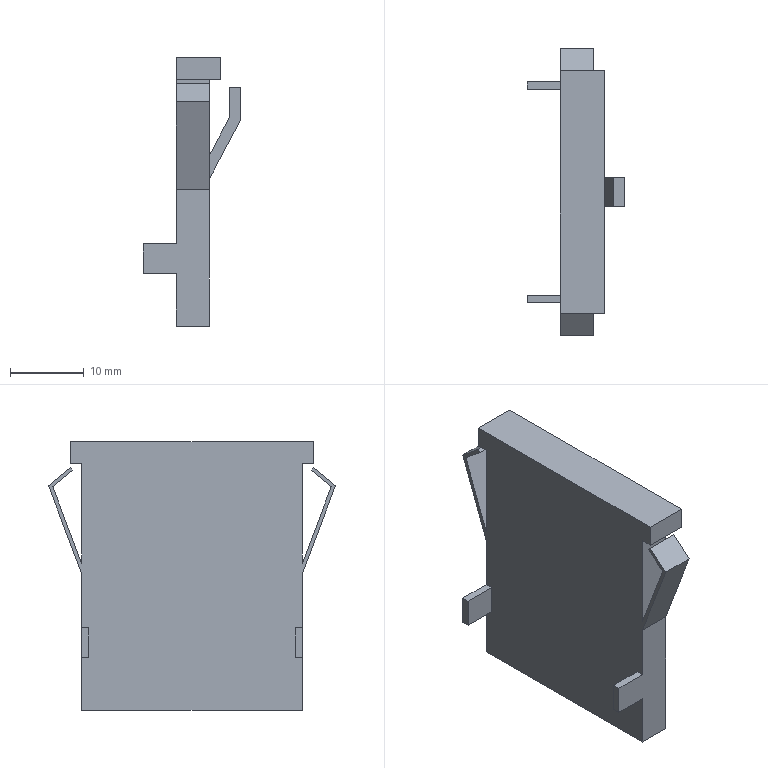Part | STEP file | A7P_M_RIGHT | 1 solid | 37 faces | box 13.3 x 39 x 36.5 mm | volume 5293 mm3 | plane 37
STEP:
#1=CARTESIAN_POINT('',(4.5,-15.,-14.9));
#2=VERTEX_POINT('',#1);
#3=CARTESIAN_POINT('',(4.5,-15.,-33.5));
#4=VERTEX_POINT('',#3);
#5=CARTESIAN_POINT('',(4.5,-15.,0.));
#6=DIRECTION('',(0.,0.,-1.));
#7=VECTOR('',#6,1000.);
#8=LINE('',#5,#7);
#9=EDGE_CURVE('',#2,#4,#8,.T.);
#10=ORIENTED_EDGE('',*,*,#9,.F.);
#11=CARTESIAN_POINT('',(0.,-15.,-14.9));
#12=VERTEX_POINT('',#11);
#13=CARTESIAN_POINT('',(0.,-15.,-14.9));
#14=DIRECTION('',(1.,0.,0.));
#15=VECTOR('',#14,1000.);
#16=LINE('',#13,#15);
#17=EDGE_CURVE('',#12,#2,#16,.T.);
#18=ORIENTED_EDGE('',*,*,#17,.F.);
#19=CARTESIAN_POINT('',(0.,-15.,-22.3));
#20=VERTEX_POINT('',#19);
#21=CARTESIAN_POINT('',(0.,-15.,0.));
#22=DIRECTION('',(0.,0.,-1.));
#23=VECTOR('',#22,1000.);
#24=LINE('',#21,#23);
#25=EDGE_CURVE('',#12,#20,#24,.T.);
#26=ORIENTED_EDGE('',*,*,#25,.T.);
#27=CARTESIAN_POINT('',(-4.5,-15.,-22.3));
#28=VERTEX_POINT('',#27);
#29=CARTESIAN_POINT('',(-4.5,-15.,-22.3));
#30=DIRECTION('',(1.,0.,0.));
#31=VECTOR('',#30,1000.);
#32=LINE('',#29,#31);
#33=EDGE_CURVE('',#28,#20,#32,.T.);
#34=ORIENTED_EDGE('',*,*,#33,.F.);
#35=CARTESIAN_POINT('',(-4.5,-15.,-26.3));
#36=VERTEX_POINT('',#35);
#37=CARTESIAN_POINT('',(-4.5,-15.,-22.3));
#38=DIRECTION('',(0.,0.,-1.));
#39=VECTOR('',#38,1000.);
#40=LINE('',#37,#39);
#41=EDGE_CURVE('',#28,#36,#40,.T.);
#42=ORIENTED_EDGE('',*,*,#41,.T.);
#43=CARTESIAN_POINT('',(0.,-15.,-26.3));
#44=VERTEX_POINT('',#43);
#45=CARTESIAN_POINT('',(-4.5,-15.,-26.3));
#46=DIRECTION('',(1.,0.,0.));
#47=VECTOR('',#46,1000.);
#48=LINE('',#45,#47);
#49=EDGE_CURVE('',#36,#44,#48,.T.);
#50=ORIENTED_EDGE('',*,*,#49,.T.);
#51=CARTESIAN_POINT('',(0.,-15.,-33.5));
#52=VERTEX_POINT('',#51);
#53=CARTESIAN_POINT('',(0.,-15.,0.));
#54=DIRECTION('',(0.,0.,-1.));
#55=VECTOR('',#54,1000.);
#56=LINE('',#53,#55);
#57=EDGE_CURVE('',#44,#52,#56,.T.);
#58=ORIENTED_EDGE('',*,*,#57,.T.);
#59=CARTESIAN_POINT('',(4.5,-15.,-33.5));
#60=DIRECTION('',(-1.,0.,0.));
#61=VECTOR('',#60,1000.);
#62=LINE('',#59,#61);
#63=EDGE_CURVE('',#4,#52,#62,.T.);
#64=ORIENTED_EDGE('',*,*,#63,.F.);
#65=EDGE_LOOP('',(#10,#18,#26,#34,#42,#50,#58,#64));
#66=FACE_OUTER_BOUND('',#65,.T.);
#67=CARTESIAN_POINT('',(4.5,-15.,0.));
#68=DIRECTION('',(0.,1.,0.));
#69=DIRECTION('',(0.,0.,1.));
#70=AXIS2_PLACEMENT_3D('',#67,#68,#69);
#71=PLANE('',#70);
#72=ADVANCED_FACE('',(#66),#71,.F.);
#73=CARTESIAN_POINT('',(0.,15.,-33.5));
#74=VERTEX_POINT('',#73);
#75=CARTESIAN_POINT('',(0.,15.,-26.3));
#76=VERTEX_POINT('',#75);
#77=CARTESIAN_POINT('',(0.,15.,0.));
#78=DIRECTION('',(0.,0.,1.));
#79=VECTOR('',#78,1000.);
#80=LINE('',#77,#79);
#81=EDGE_CURVE('',#74,#76,#80,.T.);
#82=ORIENTED_EDGE('',*,*,#81,.T.);
#83=CARTESIAN_POINT('',(-4.5,15.,-26.3));
#84=VERTEX_POINT('',#83);
#85=CARTESIAN_POINT('',(-4.5,15.,-26.3));
#86=DIRECTION('',(1.,0.,0.));
#87=VECTOR('',#86,1000.);
#88=LINE('',#85,#87);
#89=EDGE_CURVE('',#84,#76,#88,.T.);
#90=ORIENTED_EDGE('',*,*,#89,.F.);
#91=CARTESIAN_POINT('',(-4.5,15.,-22.3));
#92=VERTEX_POINT('',#91);
#93=CARTESIAN_POINT('',(-4.5,15.,-22.3));
#94=DIRECTION('',(0.,0.,1.));
#95=VECTOR('',#94,1000.);
#96=LINE('',#93,#95);
#97=EDGE_CURVE('',#84,#92,#96,.T.);
#98=ORIENTED_EDGE('',*,*,#97,.T.);
#99=CARTESIAN_POINT('',(0.,15.,-22.3));
#100=VERTEX_POINT('',#99);
#101=CARTESIAN_POINT('',(-4.5,15.,-22.3));
#102=DIRECTION('',(1.,0.,0.));
#103=VECTOR('',#102,1000.);
#104=LINE('',#101,#103);
#105=EDGE_CURVE('',#92,#100,#104,.T.);
#106=ORIENTED_EDGE('',*,*,#105,.T.);
#107=CARTESIAN_POINT('',(0.,15.,-14.9));
#108=VERTEX_POINT('',#107);
#109=CARTESIAN_POINT('',(0.,15.,0.));
#110=DIRECTION('',(0.,0.,1.));
#111=VECTOR('',#110,1000.);
#112=LINE('',#109,#111);
#113=EDGE_CURVE('',#100,#108,#112,.T.);
#114=ORIENTED_EDGE('',*,*,#113,.T.);
#115=CARTESIAN_POINT('',(4.5,15.,-14.9));
#116=VERTEX_POINT('',#115);
#117=CARTESIAN_POINT('',(0.,15.,-14.9));
#118=DIRECTION('',(1.,0.,0.));
#119=VECTOR('',#118,1000.);
#120=LINE('',#117,#119);
#121=EDGE_CURVE('',#108,#116,#120,.T.);
#122=ORIENTED_EDGE('',*,*,#121,.T.);
#123=CARTESIAN_POINT('',(4.5,15.,-33.5));
#124=VERTEX_POINT('',#123);
#125=CARTESIAN_POINT('',(4.5,15.,0.));
#126=DIRECTION('',(0.,0.,1.));
#127=VECTOR('',#126,1000.);
#128=LINE('',#125,#127);
#129=EDGE_CURVE('',#124,#116,#128,.T.);
#130=ORIENTED_EDGE('',*,*,#129,.F.);
#131=CARTESIAN_POINT('',(4.5,15.,-33.5));
#132=DIRECTION('',(-1.,0.,0.));
#133=VECTOR('',#132,1000.);
#134=LINE('',#131,#133);
#135=EDGE_CURVE('',#124,#74,#134,.T.);
#136=ORIENTED_EDGE('',*,*,#135,.T.);
#137=EDGE_LOOP('',(#82,#90,#98,#106,#114,#122,#130,#136));
#138=FACE_OUTER_BOUND('',#137,.T.);
#139=CARTESIAN_POINT('',(4.5,15.,0.));
#140=DIRECTION('',(0.,-1.,0.));
#141=DIRECTION('',(0.,0.,-1.));
#142=AXIS2_PLACEMENT_3D('',#139,#140,#141);
#143=PLANE('',#142);
#144=ADVANCED_FACE('',(#138),#143,.F.);
#145=ORIENTED_EDGE('',*,*,#129,.T.);
#146=CARTESIAN_POINT('',(4.5,19.5,-3.));
#147=VERTEX_POINT('',#146);
#148=CARTESIAN_POINT('',(4.5,19.5,-3.));
#149=DIRECTION('',(0.,0.3537,0.9354));
#150=VECTOR('',#149,1000.);
#151=LINE('',#148,#150);
#152=EDGE_CURVE('',#116,#147,#151,.T.);
#153=ORIENTED_EDGE('',*,*,#152,.T.);
#154=CARTESIAN_POINT('',(4.5,16.5,-0.5));
#155=VERTEX_POINT('',#154);
#156=CARTESIAN_POINT('',(4.5,16.5,-0.5));
#157=DIRECTION('',(0.,-0.7682,0.6402));
#158=VECTOR('',#157,1000.);
#159=LINE('',#156,#158);
#160=EDGE_CURVE('',#147,#155,#159,.T.);
#161=ORIENTED_EDGE('',*,*,#160,.T.);
#162=CARTESIAN_POINT('',(4.5,16.18,-0.8841));
#163=VERTEX_POINT('',#162);
#164=CARTESIAN_POINT('',(4.5,16.5,-0.5));
#165=DIRECTION('',(0.,-0.6402,-0.7682));
#166=VECTOR('',#165,1000.);
#167=LINE('',#164,#166);
#168=EDGE_CURVE('',#155,#163,#167,.T.);
#169=ORIENTED_EDGE('',*,*,#168,.T.);
#170=CARTESIAN_POINT('',(4.5,18.906,-3.156));
#171=VERTEX_POINT('',#170);
#172=CARTESIAN_POINT('',(4.5,16.18,-0.8841));
#173=DIRECTION('',(0.,0.7682,-0.6402));
#174=VECTOR('',#173,1000.);
#175=LINE('',#172,#174);
#176=EDGE_CURVE('',#163,#171,#175,.T.);
#177=ORIENTED_EDGE('',*,*,#176,.T.);
#178=CARTESIAN_POINT('',(4.5,15.,-13.486));
#179=VERTEX_POINT('',#178);
#180=CARTESIAN_POINT('',(4.5,18.906,-3.156));
#181=DIRECTION('',(0.,-0.3537,-0.9354));
#182=VECTOR('',#181,1000.);
#183=LINE('',#180,#182);
#184=EDGE_CURVE('',#171,#179,#183,.T.);
#185=ORIENTED_EDGE('',*,*,#184,.T.);
#186=CARTESIAN_POINT('',(4.5,15.,0.));
#187=VERTEX_POINT('',#186);
#188=CARTESIAN_POINT('',(4.5,15.,0.));
#189=DIRECTION('',(0.,0.,1.));
#190=VECTOR('',#189,1000.);
#191=LINE('',#188,#190);
#192=EDGE_CURVE('',#179,#187,#191,.T.);
#193=ORIENTED_EDGE('',*,*,#192,.T.);
#194=CARTESIAN_POINT('',(4.5,-15.,0.));
#195=VERTEX_POINT('',#194);
#196=CARTESIAN_POINT('',(4.5,16.5,0.));
#197=DIRECTION('',(0.,-1.,0.));
#198=VECTOR('',#197,1000.);
#199=LINE('',#196,#198);
#200=EDGE_CURVE('',#187,#195,#199,.T.);
#201=ORIENTED_EDGE('',*,*,#200,.T.);
#202=CARTESIAN_POINT('',(4.5,-15.,-13.486));
#203=VERTEX_POINT('',#202);
#204=CARTESIAN_POINT('',(4.5,-15.,0.));
#205=DIRECTION('',(0.,0.,-1.));
#206=VECTOR('',#205,1000.);
#207=LINE('',#204,#206);
#208=EDGE_CURVE('',#195,#203,#207,.T.);
#209=ORIENTED_EDGE('',*,*,#208,.T.);
#210=CARTESIAN_POINT('',(4.5,-18.906,-3.156));
#211=VERTEX_POINT('',#210);
#212=CARTESIAN_POINT('',(4.5,-18.906,-3.156));
#213=DIRECTION('',(0.,-0.3537,0.9354));
#214=VECTOR('',#213,1000.);
#215=LINE('',#212,#214);
#216=EDGE_CURVE('',#203,#211,#215,.T.);
#217=ORIENTED_EDGE('',*,*,#216,.T.);
#218=CARTESIAN_POINT('',(4.5,-16.18,-0.8841));
#219=VERTEX_POINT('',#218);
#220=CARTESIAN_POINT('',(4.5,-16.18,-0.8841));
#221=DIRECTION('',(0.,0.7682,0.6402));
#222=VECTOR('',#221,1000.);
#223=LINE('',#220,#222);
#224=EDGE_CURVE('',#211,#219,#223,.T.);
#225=ORIENTED_EDGE('',*,*,#224,.T.);
#226=CARTESIAN_POINT('',(4.5,-16.5,-0.5));
#227=VERTEX_POINT('',#226);
#228=CARTESIAN_POINT('',(4.5,-16.5,-0.5));
#229=DIRECTION('',(0.,-0.6402,0.7682));
#230=VECTOR('',#229,1000.);
#231=LINE('',#228,#230);
#232=EDGE_CURVE('',#219,#227,#231,.T.);
#233=ORIENTED_EDGE('',*,*,#232,.T.);
#234=CARTESIAN_POINT('',(4.5,-19.5,-3.));
#235=VERTEX_POINT('',#234);
#236=CARTESIAN_POINT('',(4.5,-16.5,-0.5));
#237=DIRECTION('',(0.,-0.7682,-0.6402));
#238=VECTOR('',#237,1000.);
#239=LINE('',#236,#238);
#240=EDGE_CURVE('',#227,#235,#239,.T.);
#241=ORIENTED_EDGE('',*,*,#240,.T.);
#242=CARTESIAN_POINT('',(4.5,-19.5,-3.));
#243=DIRECTION('',(0.,0.3537,-0.9354));
#244=VECTOR('',#243,1000.);
#245=LINE('',#242,#244);
#246=EDGE_CURVE('',#235,#2,#245,.T.);
#247=ORIENTED_EDGE('',*,*,#246,.T.);
#248=ORIENTED_EDGE('',*,*,#9,.T.);
#249=CARTESIAN_POINT('',(4.5,15.,-33.5));
#250=DIRECTION('',(0.,1.,0.));
#251=VECTOR('',#250,1000.);
#252=LINE('',#249,#251);
#253=EDGE_CURVE('',#4,#124,#252,.T.);
#254=ORIENTED_EDGE('',*,*,#253,.T.);
#255=EDGE_LOOP('',(#145,#153,#161,#169,#177,#185,#193,#201,#209,#217,#225,#233,#241,#247,#248,#254));
#256=FACE_OUTER_BOUND('',#255,.T.);
#257=CARTESIAN_POINT('',(4.5,2.,-10.292));
#258=VERTEX_POINT('',#257);
#259=CARTESIAN_POINT('',(4.5,-2.,-10.292));
#260=VERTEX_POINT('',#259);
#261=CARTESIAN_POINT('',(4.5,2.,-10.292));
#262=DIRECTION('',(0.,-1.,0.));
#263=VECTOR('',#262,1000.);
#264=LINE('',#261,#263);
#265=EDGE_CURVE('',#258,#260,#264,.T.);
#266=ORIENTED_EDGE('',*,*,#265,.F.);
#267=CARTESIAN_POINT('',(4.5,2.,-13.5));
#268=VERTEX_POINT('',#267);
#269=CARTESIAN_POINT('',(4.5,2.,-10.292));
#270=DIRECTION('',(0.,0.,1.));
#271=VECTOR('',#270,1000.);
#272=LINE('',#269,#271);
#273=EDGE_CURVE('',#268,#258,#272,.T.);
#274=ORIENTED_EDGE('',*,*,#273,.F.);
#275=CARTESIAN_POINT('',(4.5,-2.,-13.5));
#276=VERTEX_POINT('',#275);
#277=CARTESIAN_POINT('',(4.5,2.,-13.5));
#278=DIRECTION('',(0.,-1.,0.));
#279=VECTOR('',#278,1000.);
#280=LINE('',#277,#279);
#281=EDGE_CURVE('',#268,#276,#280,.T.);
#282=ORIENTED_EDGE('',*,*,#281,.T.);
#283=CARTESIAN_POINT('',(4.5,-2.,-10.292));
#284=DIRECTION('',(0.,0.,1.));
#285=VECTOR('',#284,1000.);
#286=LINE('',#283,#285);
#287=EDGE_CURVE('',#276,#260,#286,.T.);
#288=ORIENTED_EDGE('',*,*,#287,.T.);
#289=EDGE_LOOP('',(#266,#274,#282,#288));
#290=FACE_BOUND('',#289,.T.);
#291=CARTESIAN_POINT('',(4.5,16.5,0.));
#292=DIRECTION('',(1.,0.,0.));
#293=DIRECTION('',(0.,0.,-1.));
#294=AXIS2_PLACEMENT_3D('',#291,#292,#293);
#295=PLANE('',#294);
#296=ADVANCED_FACE('',(#256,#290),#295,.T.);
#297=CARTESIAN_POINT('',(0.,16.5,0.));
#298=VERTEX_POINT('',#297);
#299=CARTESIAN_POINT('',(0.,16.5,3.));
#300=VERTEX_POINT('',#299);
#301=CARTESIAN_POINT('',(0.,16.5,0.));
#302=DIRECTION('',(0.,0.,1.));
#303=VECTOR('',#302,1000.);
#304=LINE('',#301,#303);
#305=EDGE_CURVE('',#298,#300,#304,.T.);
#306=ORIENTED_EDGE('',*,*,#305,.T.);
#307=CARTESIAN_POINT('',(6.,16.5,3.));
#308=VERTEX_POINT('',#307);
#309=CARTESIAN_POINT('',(4.5,16.5,3.));
#310=DIRECTION('',(-1.,0.,0.));
#311=VECTOR('',#310,1000.);
#312=LINE('',#309,#311);
#313=EDGE_CURVE('',#308,#300,#312,.T.);
#314=ORIENTED_EDGE('',*,*,#313,.F.);
#315=CARTESIAN_POINT('',(6.,16.5,0.));
#316=VERTEX_POINT('',#315);
#317=CARTESIAN_POINT('',(6.,16.5,-33.541));
#318=DIRECTION('',(0.,0.,1.));
#319=VECTOR('',#318,1000.);
#320=LINE('',#317,#319);
#321=EDGE_CURVE('',#316,#308,#320,.T.);
#322=ORIENTED_EDGE('',*,*,#321,.F.);
#323=CARTESIAN_POINT('',(4.5,16.5,0.));
#324=DIRECTION('',(-1.,0.,0.));
#325=VECTOR('',#324,1000.);
#326=LINE('',#323,#325);
#327=EDGE_CURVE('',#316,#298,#326,.T.);
#328=ORIENTED_EDGE('',*,*,#327,.T.);
#329=EDGE_LOOP('',(#306,#314,#322,#328));
#330=FACE_OUTER_BOUND('',#329,.T.);
#331=CARTESIAN_POINT('',(4.5,16.5,0.));
#332=DIRECTION('',(0.,-1.,0.));
#333=DIRECTION('',(0.,0.,-1.));
#334=AXIS2_PLACEMENT_3D('',#331,#332,#333);
#335=PLANE('',#334);
#336=ADVANCED_FACE('',(#330),#335,.F.);
#337=CARTESIAN_POINT('',(0.,-16.5,3.));
#338=VERTEX_POINT('',#337);
#339=CARTESIAN_POINT('',(0.,16.5,3.));
#340=DIRECTION('',(0.,-1.,0.));
#341=VECTOR('',#340,1000.);
#342=LINE('',#339,#341);
#343=EDGE_CURVE('',#300,#338,#342,.T.);
#344=ORIENTED_EDGE('',*,*,#343,.T.);
#345=CARTESIAN_POINT('',(6.,-16.5,3.));
#346=VERTEX_POINT('',#345);
#347=CARTESIAN_POINT('',(4.5,-16.5,3.));
#348=DIRECTION('',(-1.,0.,0.));
#349=VECTOR('',#348,1000.);
#350=LINE('',#347,#349);
#351=EDGE_CURVE('',#346,#338,#350,.T.);
#352=ORIENTED_EDGE('',*,*,#351,.F.);
#353=CARTESIAN_POINT('',(6.,16.5,3.));
#354=DIRECTION('',(0.,1.,0.));
#355=VECTOR('',#354,1000.);
#356=LINE('',#353,#355);
#357=EDGE_CURVE('',#346,#308,#356,.T.);
#358=ORIENTED_EDGE('',*,*,#357,.T.);
#359=ORIENTED_EDGE('',*,*,#313,.T.);
#360=EDGE_LOOP('',(#344,#352,#358,#359));
#361=FACE_OUTER_BOUND('',#360,.T.);
#362=CARTESIAN_POINT('',(4.5,16.5,3.));
#363=DIRECTION('',(0.,0.,-1.));
#364=DIRECTION('',(-1.,0.,0.));
#365=AXIS2_PLACEMENT_3D('',#362,#363,#364);
#366=PLANE('',#365);
#367=ADVANCED_FACE('',(#361),#366,.F.);
#368=CARTESIAN_POINT('',(0.,-16.5,0.));
#369=VERTEX_POINT('',#368);
#370=CARTESIAN_POINT('',(0.,-16.5,3.));
#371=DIRECTION('',(0.,0.,-1.));
#372=VECTOR('',#371,1000.);
#373=LINE('',#370,#372);
#374=EDGE_CURVE('',#338,#369,#373,.T.);
#375=ORIENTED_EDGE('',*,*,#374,.T.);
#376=CARTESIAN_POINT('',(6.,-16.5,0.));
#377=VERTEX_POINT('',#376);
#378=CARTESIAN_POINT('',(4.5,-16.5,0.));
#379=DIRECTION('',(-1.,0.,0.));
#380=VECTOR('',#379,1000.);
#381=LINE('',#378,#380);
#382=EDGE_CURVE('',#377,#369,#381,.T.);
#383=ORIENTED_EDGE('',*,*,#382,.F.);
#384=CARTESIAN_POINT('',(6.,-16.5,-33.541));
#385=DIRECTION('',(0.,0.,1.));
#386=VECTOR('',#385,1000.);
#387=LINE('',#384,#386);
#388=EDGE_CURVE('',#377,#346,#387,.T.);
#389=ORIENTED_EDGE('',*,*,#388,.T.);
#390=ORIENTED_EDGE('',*,*,#351,.T.);
#391=EDGE_LOOP('',(#375,#383,#389,#390));
#392=FACE_OUTER_BOUND('',#391,.T.);
#393=CARTESIAN_POINT('',(4.5,-16.5,3.));
#394=DIRECTION('',(0.,1.,0.));
#395=DIRECTION('',(0.,0.,1.));
#396=AXIS2_PLACEMENT_3D('',#393,#394,#395);
#397=PLANE('',#396);
#398=ADVANCED_FACE('',(#392),#397,.F.);
#399=CARTESIAN_POINT('',(0.,-15.,0.));
#400=VERTEX_POINT('',#399);
#401=CARTESIAN_POINT('',(0.,-16.5,0.));
#402=DIRECTION('',(0.,1.,0.));
#403=VECTOR('',#402,1000.);
#404=LINE('',#401,#403);
#405=EDGE_CURVE('',#369,#400,#404,.T.);
#406=ORIENTED_EDGE('',*,*,#405,.T.);
#407=CARTESIAN_POINT('',(4.5,-15.,0.));
#408=DIRECTION('',(-1.,0.,0.));
#409=VECTOR('',#408,1000.);
#410=LINE('',#407,#409);
#411=EDGE_CURVE('',#195,#400,#410,.T.);
#412=ORIENTED_EDGE('',*,*,#411,.F.);
#413=ORIENTED_EDGE('',*,*,#200,.F.);
#414=CARTESIAN_POINT('',(0.,15.,0.));
#415=VERTEX_POINT('',#414);
#416=CARTESIAN_POINT('',(4.5,15.,0.));
#417=DIRECTION('',(-1.,0.,0.));
#418=VECTOR('',#417,1000.);
#419=LINE('',#416,#418);
#420=EDGE_CURVE('',#187,#415,#419,.T.);
#421=ORIENTED_EDGE('',*,*,#420,.T.);
#422=CARTESIAN_POINT('',(0.,15.,0.));
#423=DIRECTION('',(0.,1.,0.));
#424=VECTOR('',#423,1000.);
#425=LINE('',#422,#424);
#426=EDGE_CURVE('',#415,#298,#425,.T.);
#427=ORIENTED_EDGE('',*,*,#426,.T.);
#428=ORIENTED_EDGE('',*,*,#327,.F.);
#429=CARTESIAN_POINT('',(6.,16.5,0.));
#430=DIRECTION('',(0.,-1.,0.));
#431=VECTOR('',#430,1000.);
#432=LINE('',#429,#431);
#433=EDGE_CURVE('',#316,#377,#432,.T.);
#434=ORIENTED_EDGE('',*,*,#433,.T.);
#435=ORIENTED_EDGE('',*,*,#382,.T.);
#436=EDGE_LOOP('',(#406,#412,#413,#421,#427,#428,#434,#435));
#437=FACE_OUTER_BOUND('',#436,.T.);
#438=CARTESIAN_POINT('',(4.5,-16.5,0.));
#439=DIRECTION('',(0.,0.,1.));
#440=DIRECTION('',(1.,0.,0.));
#441=AXIS2_PLACEMENT_3D('',#438,#439,#440);
#442=PLANE('',#441);
#443=ADVANCED_FACE('',(#437),#442,.F.);
#444=CARTESIAN_POINT('',(0.,-15.,-13.486));
#445=VERTEX_POINT('',#444);
#446=CARTESIAN_POINT('',(0.,-15.,0.));
#447=DIRECTION('',(0.,0.,-1.));
#448=VECTOR('',#447,1000.);
#449=LINE('',#446,#448);
#450=EDGE_CURVE('',#400,#445,#449,.T.);
#451=ORIENTED_EDGE('',*,*,#450,.T.);
#452=CARTESIAN_POINT('',(0.,-15.,-13.486));
#453=DIRECTION('',(1.,0.,0.));
#454=VECTOR('',#453,1000.);
#455=LINE('',#452,#454);
#456=EDGE_CURVE('',#445,#203,#455,.T.);
#457=ORIENTED_EDGE('',*,*,#456,.T.);
#458=ORIENTED_EDGE('',*,*,#208,.F.);
#459=ORIENTED_EDGE('',*,*,#411,.T.);
#460=EDGE_LOOP('',(#451,#457,#458,#459));
#461=FACE_OUTER_BOUND('',#460,.T.);
#462=CARTESIAN_POINT('',(4.5,-15.,0.));
#463=DIRECTION('',(0.,1.,0.));
#464=DIRECTION('',(0.,0.,1.));
#465=AXIS2_PLACEMENT_3D('',#462,#463,#464);
#466=PLANE('',#465);
#467=ADVANCED_FACE('',(#461),#466,.F.);
#468=CARTESIAN_POINT('',(0.,15.,-33.5));
#469=DIRECTION('',(0.,1.,0.));
#470=VECTOR('',#469,1000.);
#471=LINE('',#468,#470);
#472=EDGE_CURVE('',#52,#74,#471,.T.);
#473=ORIENTED_EDGE('',*,*,#472,.T.);
#474=ORIENTED_EDGE('',*,*,#135,.F.);
#475=ORIENTED_EDGE('',*,*,#253,.F.);
#476=ORIENTED_EDGE('',*,*,#63,.T.);
#477=EDGE_LOOP('',(#473,#474,#475,#476));
#478=FACE_OUTER_BOUND('',#477,.T.);
#479=CARTESIAN_POINT('',(4.5,15.,-33.5));
#480=DIRECTION('',(0.,0.,1.));
#481=DIRECTION('',(1.,0.,0.));
#482=AXIS2_PLACEMENT_3D('',#479,#480,#481);
#483=PLANE('',#482);
#484=ADVANCED_FACE('',(#478),#483,.F.);
#485=ORIENTED_EDGE('',*,*,#192,.F.);
#486=CARTESIAN_POINT('',(0.,15.,-13.486));
#487=VERTEX_POINT('',#486);
#488=CARTESIAN_POINT('',(0.,15.,-13.486));
#489=DIRECTION('',(1.,0.,0.));
#490=VECTOR('',#489,1000.);
#491=LINE('',#488,#490);
#492=EDGE_CURVE('',#487,#179,#491,.T.);
#493=ORIENTED_EDGE('',*,*,#492,.F.);
#494=CARTESIAN_POINT('',(0.,15.,0.));
#495=DIRECTION('',(0.,0.,1.));
#496=VECTOR('',#495,1000.);
#497=LINE('',#494,#496);
#498=EDGE_CURVE('',#487,#415,#497,.T.);
#499=ORIENTED_EDGE('',*,*,#498,.T.);
#500=ORIENTED_EDGE('',*,*,#420,.F.);
#501=EDGE_LOOP('',(#485,#493,#499,#500));
#502=FACE_OUTER_BOUND('',#501,.T.);
#503=CARTESIAN_POINT('',(4.5,15.,0.));
#504=DIRECTION('',(0.,-1.,0.));
#505=DIRECTION('',(0.,0.,-1.));
#506=AXIS2_PLACEMENT_3D('',#503,#504,#505);
#507=PLANE('',#506);
#508=ADVANCED_FACE('',(#502),#507,.F.);
#509=CARTESIAN_POINT('',(0.,-14.,-26.3));
#510=VERTEX_POINT('',#509);
#511=CARTESIAN_POINT('',(0.,-14.,-22.3));
#512=VERTEX_POINT('',#511);
#513=CARTESIAN_POINT('',(0.,-14.,-22.3));
#514=DIRECTION('',(0.,0.,1.));
#515=VECTOR('',#514,1000.);
#516=LINE('',#513,#515);
#517=EDGE_CURVE('',#510,#512,#516,.T.);
#518=ORIENTED_EDGE('',*,*,#517,.T.);
#519=CARTESIAN_POINT('',(0.,-15.,-22.3));
#520=DIRECTION('',(0.,-1.,0.));
#521=VECTOR('',#520,1000.);
#522=LINE('',#519,#521);
#523=EDGE_CURVE('',#512,#20,#522,.T.);
#524=ORIENTED_EDGE('',*,*,#523,.T.);
#525=ORIENTED_EDGE('',*,*,#25,.F.);
#526=CARTESIAN_POINT('',(0.,-19.5,-3.));
#527=VERTEX_POINT('',#526);
#528=CARTESIAN_POINT('',(0.,-19.5,-3.));
#529=DIRECTION('',(0.,0.3537,-0.9354));
#530=VECTOR('',#529,1000.);
#531=LINE('',#528,#530);
#532=EDGE_CURVE('',#527,#12,#531,.T.);
#533=ORIENTED_EDGE('',*,*,#532,.F.);
#534=CARTESIAN_POINT('',(0.,-16.5,-0.5));
#535=VERTEX_POINT('',#534);
#536=CARTESIAN_POINT('',(0.,-16.5,-0.5));
#537=DIRECTION('',(0.,-0.7682,-0.6402));
#538=VECTOR('',#537,1000.);
#539=LINE('',#536,#538);
#540=EDGE_CURVE('',#535,#527,#539,.T.);
#541=ORIENTED_EDGE('',*,*,#540,.F.);
#542=CARTESIAN_POINT('',(0.,-16.18,-0.8841));
#543=VERTEX_POINT('',#542);
#544=CARTESIAN_POINT('',(0.,-16.5,-0.5));
#545=DIRECTION('',(0.,-0.6402,0.7682));
#546=VECTOR('',#545,1000.);
#547=LINE('',#544,#546);
#548=EDGE_CURVE('',#543,#535,#547,.T.);
#549=ORIENTED_EDGE('',*,*,#548,.F.);
#550=CARTESIAN_POINT('',(0.,-18.906,-3.156));
#551=VERTEX_POINT('',#550);
#552=CARTESIAN_POINT('',(0.,-16.18,-0.8841));
#553=DIRECTION('',(0.,0.7682,0.6402));
#554=VECTOR('',#553,1000.);
#555=LINE('',#552,#554);
#556=EDGE_CURVE('',#551,#543,#555,.T.);
#557=ORIENTED_EDGE('',*,*,#556,.F.);
#558=CARTESIAN_POINT('',(0.,-18.906,-3.156));
#559=DIRECTION('',(0.,-0.3537,0.9354));
#560=VECTOR('',#559,1000.);
#561=LINE('',#558,#560);
#562=EDGE_CURVE('',#445,#551,#561,.T.);
#563=ORIENTED_EDGE('',*,*,#562,.F.);
#564=ORIENTED_EDGE('',*,*,#450,.F.);
#565=ORIENTED_EDGE('',*,*,#405,.F.);
#566=ORIENTED_EDGE('',*,*,#374,.F.);
#567=ORIENTED_EDGE('',*,*,#343,.F.);
#568=ORIENTED_EDGE('',*,*,#305,.F.);
#569=ORIENTED_EDGE('',*,*,#426,.F.);
#570=ORIENTED_EDGE('',*,*,#498,.F.);
#571=CARTESIAN_POINT('',(0.,18.906,-3.156));
#572=VERTEX_POINT('',#571);
#573=CARTESIAN_POINT('',(0.,18.906,-3.156));
#574=DIRECTION('',(0.,-0.3537,-0.9354));
#575=VECTOR('',#574,1000.);
#576=LINE('',#573,#575);
#577=EDGE_CURVE('',#572,#487,#576,.T.);
#578=ORIENTED_EDGE('',*,*,#577,.F.);
#579=CARTESIAN_POINT('',(0.,16.18,-0.8841));
#580=VERTEX_POINT('',#579);
#581=CARTESIAN_POINT('',(0.,16.18,-0.8841));
#582=DIRECTION('',(0.,0.7682,-0.6402));
#583=VECTOR('',#582,1000.);
#584=LINE('',#581,#583);
#585=EDGE_CURVE('',#580,#572,#584,.T.);
#586=ORIENTED_EDGE('',*,*,#585,.F.);
#587=CARTESIAN_POINT('',(0.,16.5,-0.5));
#588=VERTEX_POINT('',#587);
#589=CARTESIAN_POINT('',(0.,16.5,-0.5));
#590=DIRECTION('',(0.,-0.6402,-0.7682));
#591=VECTOR('',#590,1000.);
#592=LINE('',#589,#591);
#593=EDGE_CURVE('',#588,#580,#592,.T.);
#594=ORIENTED_EDGE('',*,*,#593,.F.);
#595=CARTESIAN_POINT('',(0.,19.5,-3.));
#596=VERTEX_POINT('',#595);
#597=CARTESIAN_POINT('',(0.,16.5,-0.5));
#598=DIRECTION('',(0.,-0.7682,0.6402));
#599=VECTOR('',#598,1000.);
#600=LINE('',#597,#599);
#601=EDGE_CURVE('',#596,#588,#600,.T.);
#602=ORIENTED_EDGE('',*,*,#601,.F.);
#603=CARTESIAN_POINT('',(0.,19.5,-3.));
#604=DIRECTION('',(0.,0.3537,0.9354));
#605=VECTOR('',#604,1000.);
#606=LINE('',#603,#605);
#607=EDGE_CURVE('',#108,#596,#606,.T.);
#608=ORIENTED_EDGE('',*,*,#607,.F.);
#609=ORIENTED_EDGE('',*,*,#113,.F.);
#610=CARTESIAN_POINT('',(0.,14.,-22.3));
#611=VERTEX_POINT('',#610);
#612=CARTESIAN_POINT('',(0.,15.,-22.3));
#613=DIRECTION('',(0.,-1.,0.));
#614=VECTOR('',#613,1000.);
#615=LINE('',#612,#614);
#616=EDGE_CURVE('',#100,#611,#615,.T.);
#617=ORIENTED_EDGE('',*,*,#616,.T.);
#618=CARTESIAN_POINT('',(0.,14.,-26.3));
#619=VERTEX_POINT('',#618);
#620=CARTESIAN_POINT('',(0.,14.,-22.3));
#621=DIRECTION('',(0.,0.,-1.));
#622=VECTOR('',#621,1000.);
#623=LINE('',#620,#622);
#624=EDGE_CURVE('',#611,#619,#623,.T.);
#625=ORIENTED_EDGE('',*,*,#624,.T.);
#626=CARTESIAN_POINT('',(0.,15.,-26.3));
#627=DIRECTION('',(0.,1.,0.));
#628=VECTOR('',#627,1000.);
#629=LINE('',#626,#628);
#630=EDGE_CURVE('',#619,#76,#629,.T.);
#631=ORIENTED_EDGE('',*,*,#630,.T.);
#632=ORIENTED_EDGE('',*,*,#81,.F.);
#633=ORIENTED_EDGE('',*,*,#472,.F.);
#634=ORIENTED_EDGE('',*,*,#57,.F.);
#635=CARTESIAN_POINT('',(0.,-15.,-26.3));
#636=DIRECTION('',(0.,1.,0.));
#637=VECTOR('',#636,1000.);
#638=LINE('',#635,#637);
#639=EDGE_CURVE('',#44,#510,#638,.T.);
#640=ORIENTED_EDGE('',*,*,#639,.T.);
#641=EDGE_LOOP('',(#518,#524,#525,#533,#541,#549,#557,#563,#564,#565,#566,#567,#568,#569,#570,#578,#586,#594,#602,#608,#609,#617,#625,#631,#632,#633,#634,#640));
#642=FACE_OUTER_BOUND('',#641,.T.);
#643=CARTESIAN_POINT('',(0.,16.5,0.));
#644=DIRECTION('',(1.,0.,0.));
#645=DIRECTION('',(0.,0.,-1.));
#646=AXIS2_PLACEMENT_3D('',#643,#644,#645);
#647=PLANE('',#646);
#648=ADVANCED_FACE('',(#642),#647,.F.);
#649=ORIENTED_EDGE('',*,*,#433,.F.);
#650=ORIENTED_EDGE('',*,*,#321,.T.);
#651=ORIENTED_EDGE('',*,*,#357,.F.);
#652=ORIENTED_EDGE('',*,*,#388,.F.);
#653=EDGE_LOOP('',(#649,#650,#651,#652));
#654=FACE_OUTER_BOUND('',#653,.T.);
#655=CARTESIAN_POINT('',(6.,16.5,-33.541));
#656=DIRECTION('',(1.,0.,0.));
#657=DIRECTION('',(0.,1.,0.));
#658=AXIS2_PLACEMENT_3D('',#655,#656,#657);
#659=PLANE('',#658);
#660=ADVANCED_FACE('',(#654),#659,.T.);
#661=CARTESIAN_POINT('',(7.3,-2.,-5.));
#662=VERTEX_POINT('',#661);
#663=CARTESIAN_POINT('',(4.5,-2.,-10.292));
#664=DIRECTION('',(0.4676,0.,0.8839));
#665=VECTOR('',#664,1000.);
#666=LINE('',#663,#665);
#667=EDGE_CURVE('',#260,#662,#666,.T.);
#668=ORIENTED_EDGE('',*,*,#667,.T.);
#669=CARTESIAN_POINT('',(7.3,2.,-5.));
#670=VERTEX_POINT('',#669);
#671=CARTESIAN_POINT('',(7.3,2.,-5.));
#672=DIRECTION('',(0.,-1.,0.));
#673=VECTOR('',#672,1000.);
#674=LINE('',#671,#673);
#675=EDGE_CURVE('',#670,#662,#674,.T.);
#676=ORIENTED_EDGE('',*,*,#675,.F.);
#677=CARTESIAN_POINT('',(4.5,2.,-10.292));
#678=DIRECTION('',(0.4676,0.,0.8839));
#679=VECTOR('',#678,1000.);
#680=LINE('',#677,#679);
#681=EDGE_CURVE('',#258,#670,#680,.T.);
#682=ORIENTED_EDGE('',*,*,#681,.F.);
#683=ORIENTED_EDGE('',*,*,#265,.T.);
#684=EDGE_LOOP('',(#668,#676,#682,#683));
#685=FACE_OUTER_BOUND('',#684,.T.);
#686=CARTESIAN_POINT('',(4.5,2.,-10.292));
#687=DIRECTION('',(0.8839,0.,-0.4676));
#688=DIRECTION('',(-0.4676,0.,-0.8839));
#689=AXIS2_PLACEMENT_3D('',#686,#687,#688);
#690=PLANE('',#689);
#691=ADVANCED_FACE('',(#685),#690,.F.);
#692=CARTESIAN_POINT('',(7.3,-2.,-1.));
#693=VERTEX_POINT('',#692);
#694=CARTESIAN_POINT('',(7.3,-2.,-5.));
#695=DIRECTION('',(0.,0.,1.));
#696=VECTOR('',#695,1000.);
#697=LINE('',#694,#696);
#698=EDGE_CURVE('',#662,#693,#697,.T.);
#699=ORIENTED_EDGE('',*,*,#698,.T.);
#700=CARTESIAN_POINT('',(7.3,2.,-1.));
#701=VERTEX_POINT('',#700);
#702=CARTESIAN_POINT('',(7.3,2.,-1.));
#703=DIRECTION('',(0.,-1.,0.));
#704=VECTOR('',#703,1000.);
#705=LINE('',#702,#704);
#706=EDGE_CURVE('',#701,#693,#705,.T.);
#707=ORIENTED_EDGE('',*,*,#706,.F.);
#708=CARTESIAN_POINT('',(7.3,2.,-5.));
#709=DIRECTION('',(0.,0.,1.));
#710=VECTOR('',#709,1000.);
#711=LINE('',#708,#710);
#712=EDGE_CURVE('',#670,#701,#711,.T.);
#713=ORIENTED_EDGE('',*,*,#712,.F.);
#714=ORIENTED_EDGE('',*,*,#675,.T.);
#715=EDGE_LOOP('',(#699,#707,#713,#714));
#716=FACE_OUTER_BOUND('',#715,.T.);
#717=CARTESIAN_POINT('',(7.3,2.,-5.));
#718=DIRECTION('',(1.,0.,0.));
#719=DIRECTION('',(0.,0.,-1.));
#720=AXIS2_PLACEMENT_3D('',#717,#718,#719);
#721=PLANE('',#720);
#722=ADVANCED_FACE('',(#716),#721,.F.);
#723=CARTESIAN_POINT('',(8.8,-2.,-1.));
#724=VERTEX_POINT('',#723);
#725=CARTESIAN_POINT('',(7.3,-2.,-1.));
#726=DIRECTION('',(1.,0.,0.));
#727=VECTOR('',#726,1000.);
#728=LINE('',#725,#727);
#729=EDGE_CURVE('',#693,#724,#728,.T.);
#730=ORIENTED_EDGE('',*,*,#729,.T.);
#731=CARTESIAN_POINT('',(8.8,2.,-1.));
#732=VERTEX_POINT('',#731);
#733=CARTESIAN_POINT('',(8.8,2.,-1.));
#734=DIRECTION('',(0.,-1.,0.));
#735=VECTOR('',#734,1000.);
#736=LINE('',#733,#735);
#737=EDGE_CURVE('',#732,#724,#736,.T.);
#738=ORIENTED_EDGE('',*,*,#737,.F.);
#739=CARTESIAN_POINT('',(7.3,2.,-1.));
#740=DIRECTION('',(1.,0.,0.));
#741=VECTOR('',#740,1000.);
#742=LINE('',#739,#741);
#743=EDGE_CURVE('',#701,#732,#742,.T.);
#744=ORIENTED_EDGE('',*,*,#743,.F.);
#745=ORIENTED_EDGE('',*,*,#706,.T.);
#746=EDGE_LOOP('',(#730,#738,#744,#745));
#747=FACE_OUTER_BOUND('',#746,.T.);
#748=CARTESIAN_POINT('',(7.3,2.,-1.));
#749=DIRECTION('',(0.,0.,-1.));
#750=DIRECTION('',(-1.,0.,0.));
#751=AXIS2_PLACEMENT_3D('',#748,#749,#750);
#752=PLANE('',#751);
#753=ADVANCED_FACE('',(#747),#752,.F.);
#754=CARTESIAN_POINT('',(8.8,-2.,-5.372));
#755=VERTEX_POINT('',#754);
#756=CARTESIAN_POINT('',(8.8,-2.,-5.372));
#757=DIRECTION('',(0.,0.,-1.));
#758=VECTOR('',#757,1000.);
#759=LINE('',#756,#758);
#760=EDGE_CURVE('',#724,#755,#759,.T.);
#761=ORIENTED_EDGE('',*,*,#760,.T.);
#762=CARTESIAN_POINT('',(8.8,2.,-5.372));
#763=VERTEX_POINT('',#762);
#764=CARTESIAN_POINT('',(8.8,2.,-5.372));
#765=DIRECTION('',(0.,-1.,0.));
#766=VECTOR('',#765,1000.);
#767=LINE('',#764,#766);
#768=EDGE_CURVE('',#763,#755,#767,.T.);
#769=ORIENTED_EDGE('',*,*,#768,.F.);
#770=CARTESIAN_POINT('',(8.8,2.,-5.372));
#771=DIRECTION('',(0.,0.,-1.));
#772=VECTOR('',#771,1000.);
#773=LINE('',#770,#772);
#774=EDGE_CURVE('',#732,#763,#773,.T.);
#775=ORIENTED_EDGE('',*,*,#774,.F.);
#776=ORIENTED_EDGE('',*,*,#737,.T.);
#777=EDGE_LOOP('',(#761,#769,#775,#776));
#778=FACE_OUTER_BOUND('',#777,.T.);
#779=CARTESIAN_POINT('',(8.8,2.,-5.372));
#780=DIRECTION('',(-1.,0.,0.));
#781=DIRECTION('',(0.,0.,1.));
#782=AXIS2_PLACEMENT_3D('',#779,#780,#781);
#783=PLANE('',#782);
#784=ADVANCED_FACE('',(#778),#783,.F.);
#785=CARTESIAN_POINT('',(4.5,-2.,-13.5));
#786=DIRECTION('',(-0.4676,0.,-0.8839));
#787=VECTOR('',#786,1000.);
#788=LINE('',#785,#787);
#789=EDGE_CURVE('',#755,#276,#788,.T.);
#790=ORIENTED_EDGE('',*,*,#789,.T.);
#791=ORIENTED_EDGE('',*,*,#281,.F.);
#792=CARTESIAN_POINT('',(4.5,2.,-13.5));
#793=DIRECTION('',(-0.4676,0.,-0.8839));
#794=VECTOR('',#793,1000.);
#795=LINE('',#792,#794);
#796=EDGE_CURVE('',#763,#268,#795,.T.);
#797=ORIENTED_EDGE('',*,*,#796,.F.);
#798=ORIENTED_EDGE('',*,*,#768,.T.);
#799=EDGE_LOOP('',(#790,#791,#797,#798));
#800=FACE_OUTER_BOUND('',#799,.T.);
#801=CARTESIAN_POINT('',(4.5,2.,-13.5));
#802=DIRECTION('',(-0.8839,0.,0.4676));
#803=DIRECTION('',(0.4676,0.,0.8839));
#804=AXIS2_PLACEMENT_3D('',#801,#802,#803);
#805=PLANE('',#804);
#806=ADVANCED_FACE('',(#800),#805,.F.);
#807=ORIENTED_EDGE('',*,*,#273,.T.);
#808=ORIENTED_EDGE('',*,*,#681,.T.);
#809=ORIENTED_EDGE('',*,*,#712,.T.);
#810=ORIENTED_EDGE('',*,*,#743,.T.);
#811=ORIENTED_EDGE('',*,*,#774,.T.);
#812=ORIENTED_EDGE('',*,*,#796,.T.);
#813=EDGE_LOOP('',(#807,#808,#809,#810,#811,#812));
#814=FACE_OUTER_BOUND('',#813,.T.);
#815=CARTESIAN_POINT('',(4.5,2.,-1.));
#816=DIRECTION('',(0.,-1.,0.));
#817=DIRECTION('',(0.,0.,-1.));
#818=AXIS2_PLACEMENT_3D('',#815,#816,#817);
#819=PLANE('',#818);
#820=ADVANCED_FACE('',(#814),#819,.F.);
#821=ORIENTED_EDGE('',*,*,#287,.F.);
#822=ORIENTED_EDGE('',*,*,#789,.F.);
#823=ORIENTED_EDGE('',*,*,#760,.F.);
#824=ORIENTED_EDGE('',*,*,#729,.F.);
#825=ORIENTED_EDGE('',*,*,#698,.F.);
#826=ORIENTED_EDGE('',*,*,#667,.F.);
#827=EDGE_LOOP('',(#821,#822,#823,#824,#825,#826));
#828=FACE_OUTER_BOUND('',#827,.T.);
#829=CARTESIAN_POINT('',(4.5,-2.,-1.));
#830=DIRECTION('',(0.,-1.,0.));
#831=DIRECTION('',(0.,0.,-1.));
#832=AXIS2_PLACEMENT_3D('',#829,#830,#831);
#833=PLANE('',#832);
#834=ADVANCED_FACE('',(#828),#833,.T.);
#835=ORIENTED_EDGE('',*,*,#168,.F.);
#836=CARTESIAN_POINT('',(0.,16.5,-0.5));
#837=DIRECTION('',(1.,0.,0.));
#838=VECTOR('',#837,1000.);
#839=LINE('',#836,#838);
#840=EDGE_CURVE('',#588,#155,#839,.T.);
#841=ORIENTED_EDGE('',*,*,#840,.F.);
#842=ORIENTED_EDGE('',*,*,#593,.T.);
#843=CARTESIAN_POINT('',(0.,16.18,-0.8841));
#844=DIRECTION('',(1.,0.,0.));
#845=VECTOR('',#844,1000.);
#846=LINE('',#843,#845);
#847=EDGE_CURVE('',#580,#163,#846,.T.);
#848=ORIENTED_EDGE('',*,*,#847,.T.);
#849=EDGE_LOOP('',(#835,#841,#842,#848));
#850=FACE_OUTER_BOUND('',#849,.T.);
#851=CARTESIAN_POINT('',(0.,16.5,-0.5));
#852=DIRECTION('',(0.,-0.7682,0.6402));
#853=DIRECTION('',(0.,-0.6402,-0.7682));
#854=AXIS2_PLACEMENT_3D('',#851,#852,#853);
#855=PLANE('',#854);
#856=ADVANCED_FACE('',(#850),#855,.T.);
#857=ORIENTED_EDGE('',*,*,#160,.F.);
#858=CARTESIAN_POINT('',(0.,19.5,-3.));
#859=DIRECTION('',(1.,0.,0.));
#860=VECTOR('',#859,1000.);
#861=LINE('',#858,#860);
#862=EDGE_CURVE('',#596,#147,#861,.T.);
#863=ORIENTED_EDGE('',*,*,#862,.F.);
#864=ORIENTED_EDGE('',*,*,#601,.T.);
#865=ORIENTED_EDGE('',*,*,#840,.T.);
#866=EDGE_LOOP('',(#857,#863,#864,#865));
#867=FACE_OUTER_BOUND('',#866,.T.);
#868=CARTESIAN_POINT('',(0.,16.5,-0.5));
#869=DIRECTION('',(0.,0.6402,0.7682));
#870=DIRECTION('',(0.,-0.7682,0.6402));
#871=AXIS2_PLACEMENT_3D('',#868,#869,#870);
#872=PLANE('',#871);
#873=ADVANCED_FACE('',(#867),#872,.T.);
#874=ORIENTED_EDGE('',*,*,#152,.F.);
#875=ORIENTED_EDGE('',*,*,#121,.F.);
#876=ORIENTED_EDGE('',*,*,#607,.T.);
#877=ORIENTED_EDGE('',*,*,#862,.T.);
#878=EDGE_LOOP('',(#874,#875,#876,#877));
#879=FACE_OUTER_BOUND('',#878,.T.);
#880=CARTESIAN_POINT('',(0.,19.5,-3.));
#881=DIRECTION('',(0.,0.9354,-0.3537));
#882=DIRECTION('',(0.,0.3537,0.9354));
#883=AXIS2_PLACEMENT_3D('',#880,#881,#882);
#884=PLANE('',#883);
#885=ADVANCED_FACE('',(#879),#884,.T.);
#886=ORIENTED_EDGE('',*,*,#184,.F.);
#887=CARTESIAN_POINT('',(0.,18.906,-3.156));
#888=DIRECTION('',(1.,0.,0.));
#889=VECTOR('',#888,1000.);
#890=LINE('',#887,#889);
#891=EDGE_CURVE('',#572,#171,#890,.T.);
#892=ORIENTED_EDGE('',*,*,#891,.F.);
#893=ORIENTED_EDGE('',*,*,#577,.T.);
#894=ORIENTED_EDGE('',*,*,#492,.T.);
#895=EDGE_LOOP('',(#886,#892,#893,#894));
#896=FACE_OUTER_BOUND('',#895,.T.);
#897=CARTESIAN_POINT('',(0.,18.906,-3.156));
#898=DIRECTION('',(0.,-0.9354,0.3537));
#899=DIRECTION('',(0.,-0.3537,-0.9354));
#900=AXIS2_PLACEMENT_3D('',#897,#898,#899);
#901=PLANE('',#900);
#902=ADVANCED_FACE('',(#896),#901,.T.);
#903=ORIENTED_EDGE('',*,*,#176,.F.);
#904=ORIENTED_EDGE('',*,*,#847,.F.);
#905=ORIENTED_EDGE('',*,*,#585,.T.);
#906=ORIENTED_EDGE('',*,*,#891,.T.);
#907=EDGE_LOOP('',(#903,#904,#905,#906));
#908=FACE_OUTER_BOUND('',#907,.T.);
#909=CARTESIAN_POINT('',(0.,16.18,-0.8841));
#910=DIRECTION('',(0.,-0.6402,-0.7682));
#911=DIRECTION('',(0.,0.7682,-0.6402));
#912=AXIS2_PLACEMENT_3D('',#909,#910,#911);
#913=PLANE('',#912);
#914=ADVANCED_FACE('',(#908),#913,.T.);
#915=ORIENTED_EDGE('',*,*,#246,.F.);
#916=CARTESIAN_POINT('',(0.,-19.5,-3.));
#917=DIRECTION('',(1.,0.,0.));
#918=VECTOR('',#917,1000.);
#919=LINE('',#916,#918);
#920=EDGE_CURVE('',#527,#235,#919,.T.);
#921=ORIENTED_EDGE('',*,*,#920,.F.);
#922=ORIENTED_EDGE('',*,*,#532,.T.);
#923=ORIENTED_EDGE('',*,*,#17,.T.);
#924=EDGE_LOOP('',(#915,#921,#922,#923));
#925=FACE_OUTER_BOUND('',#924,.T.);
#926=CARTESIAN_POINT('',(0.,-19.5,-3.));
#927=DIRECTION('',(0.,-0.9354,-0.3537));
#928=DIRECTION('',(0.,0.3537,-0.9354));
#929=AXIS2_PLACEMENT_3D('',#926,#927,#928);
#930=PLANE('',#929);
#931=ADVANCED_FACE('',(#925),#930,.T.);
#932=ORIENTED_EDGE('',*,*,#240,.F.);
#933=CARTESIAN_POINT('',(0.,-16.5,-0.5));
#934=DIRECTION('',(1.,0.,0.));
#935=VECTOR('',#934,1000.);
#936=LINE('',#933,#935);
#937=EDGE_CURVE('',#535,#227,#936,.T.);
#938=ORIENTED_EDGE('',*,*,#937,.F.);
#939=ORIENTED_EDGE('',*,*,#540,.T.);
#940=ORIENTED_EDGE('',*,*,#920,.T.);
#941=EDGE_LOOP('',(#932,#938,#939,#940));
#942=FACE_OUTER_BOUND('',#941,.T.);
#943=CARTESIAN_POINT('',(0.,-16.5,-0.5));
#944=DIRECTION('',(0.,-0.6402,0.7682));
#945=DIRECTION('',(0.,-0.7682,-0.6402));
#946=AXIS2_PLACEMENT_3D('',#943,#944,#945);
#947=PLANE('',#946);
#948=ADVANCED_FACE('',(#942),#947,.T.);
#949=ORIENTED_EDGE('',*,*,#232,.F.);
#950=CARTESIAN_POINT('',(0.,-16.18,-0.8841));
#951=DIRECTION('',(1.,0.,0.));
#952=VECTOR('',#951,1000.);
#953=LINE('',#950,#952);
#954=EDGE_CURVE('',#543,#219,#953,.T.);
#955=ORIENTED_EDGE('',*,*,#954,.F.);
#956=ORIENTED_EDGE('',*,*,#548,.T.);
#957=ORIENTED_EDGE('',*,*,#937,.T.);
#958=EDGE_LOOP('',(#949,#955,#956,#957));
#959=FACE_OUTER_BOUND('',#958,.T.);
#960=CARTESIAN_POINT('',(0.,-16.5,-0.5));
#961=DIRECTION('',(0.,0.7682,0.6402));
#962=DIRECTION('',(0.,-0.6402,0.7682));
#963=AXIS2_PLACEMENT_3D('',#960,#961,#962);
#964=PLANE('',#963);
#965=ADVANCED_FACE('',(#959),#964,.T.);
#966=ORIENTED_EDGE('',*,*,#224,.F.);
#967=CARTESIAN_POINT('',(0.,-18.906,-3.156));
#968=DIRECTION('',(1.,0.,0.));
#969=VECTOR('',#968,1000.);
#970=LINE('',#967,#969);
#971=EDGE_CURVE('',#551,#211,#970,.T.);
#972=ORIENTED_EDGE('',*,*,#971,.F.);
#973=ORIENTED_EDGE('',*,*,#556,.T.);
#974=ORIENTED_EDGE('',*,*,#954,.T.);
#975=EDGE_LOOP('',(#966,#972,#973,#974));
#976=FACE_OUTER_BOUND('',#975,.T.);
#977=CARTESIAN_POINT('',(0.,-16.18,-0.8841));
#978=DIRECTION('',(0.,0.6402,-0.7682));
#979=DIRECTION('',(0.,0.7682,0.6402));
#980=AXIS2_PLACEMENT_3D('',#977,#978,#979);
#981=PLANE('',#980);
#982=ADVANCED_FACE('',(#976),#981,.T.);
#983=ORIENTED_EDGE('',*,*,#216,.F.);
#984=ORIENTED_EDGE('',*,*,#456,.F.);
#985=ORIENTED_EDGE('',*,*,#562,.T.);
#986=ORIENTED_EDGE('',*,*,#971,.T.);
#987=EDGE_LOOP('',(#983,#984,#985,#986));
#988=FACE_OUTER_BOUND('',#987,.T.);
#989=CARTESIAN_POINT('',(0.,-18.906,-3.156));
#990=DIRECTION('',(0.,0.9354,0.3537));
#991=DIRECTION('',(0.,-0.3537,0.9354));
#992=AXIS2_PLACEMENT_3D('',#989,#990,#991);
#993=PLANE('',#992);
#994=ADVANCED_FACE('',(#988),#993,.T.);
#995=ORIENTED_EDGE('',*,*,#616,.F.);
#996=ORIENTED_EDGE('',*,*,#105,.F.);
#997=CARTESIAN_POINT('',(-4.5,14.,-22.3));
#998=VERTEX_POINT('',#997);
#999=CARTESIAN_POINT('',(-4.5,15.,-22.3));
#1000=DIRECTION('',(0.,-1.,0.));
#1001=VECTOR('',#1000,1000.);
#1002=LINE('',#999,#1001);
#1003=EDGE_CURVE('',#92,#998,#1002,.T.);
#1004=ORIENTED_EDGE('',*,*,#1003,.T.);
#1005=CARTESIAN_POINT('',(-4.5,14.,-22.3));
#1006=DIRECTION('',(1.,0.,0.));
#1007=VECTOR('',#1006,1000.);
#1008=LINE('',#1005,#1007);
#1009=EDGE_CURVE('',#998,#611,#1008,.T.);
#1010=ORIENTED_EDGE('',*,*,#1009,.T.);
#1011=EDGE_LOOP('',(#995,#996,#1004,#1010));
#1012=FACE_OUTER_BOUND('',#1011,.T.);
#1013=CARTESIAN_POINT('',(-4.5,15.,-22.3));
#1014=DIRECTION('',(0.,0.,1.));
#1015=DIRECTION('',(0.,-1.,0.));
#1016=AXIS2_PLACEMENT_3D('',#1013,#1014,#1015);
#1017=PLANE('',#1016);
#1018=ADVANCED_FACE('',(#1012),#1017,.T.);
#1019=ORIENTED_EDGE('',*,*,#630,.F.);
#1020=CARTESIAN_POINT('',(-4.5,14.,-26.3));
#1021=VERTEX_POINT('',#1020);
#1022=CARTESIAN_POINT('',(-4.5,14.,-26.3));
#1023=DIRECTION('',(1.,0.,0.));
#1024=VECTOR('',#1023,1000.);
#1025=LINE('',#1022,#1024);
#1026=EDGE_CURVE('',#1021,#619,#1025,.T.);
#1027=ORIENTED_EDGE('',*,*,#1026,.F.);
#1028=CARTESIAN_POINT('',(-4.5,15.,-26.3));
#1029=DIRECTION('',(0.,1.,0.));
#1030=VECTOR('',#1029,1000.);
#1031=LINE('',#1028,#1030);
#1032=EDGE_CURVE('',#1021,#84,#1031,.T.);
#1033=ORIENTED_EDGE('',*,*,#1032,.T.);
#1034=ORIENTED_EDGE('',*,*,#89,.T.);
#1035=EDGE_LOOP('',(#1019,#1027,#1033,#1034));
#1036=FACE_OUTER_BOUND('',#1035,.T.);
#1037=CARTESIAN_POINT('',(-4.5,15.,-26.3));
#1038=DIRECTION('',(0.,0.,-1.));
#1039=DIRECTION('',(0.,1.,0.));
#1040=AXIS2_PLACEMENT_3D('',#1037,#1038,#1039);
#1041=PLANE('',#1040);
#1042=ADVANCED_FACE('',(#1036),#1041,.T.);
#1043=ORIENTED_EDGE('',*,*,#624,.F.);
#1044=ORIENTED_EDGE('',*,*,#1009,.F.);
#1045=CARTESIAN_POINT('',(-4.5,14.,-22.3));
#1046=DIRECTION('',(0.,0.,-1.));
#1047=VECTOR('',#1046,1000.);
#1048=LINE('',#1045,#1047);
#1049=EDGE_CURVE('',#998,#1021,#1048,.T.);
#1050=ORIENTED_EDGE('',*,*,#1049,.T.);
#1051=ORIENTED_EDGE('',*,*,#1026,.T.);
#1052=EDGE_LOOP('',(#1043,#1044,#1050,#1051));
#1053=FACE_OUTER_BOUND('',#1052,.T.);
#1054=CARTESIAN_POINT('',(-4.5,14.,-22.3));
#1055=DIRECTION('',(0.,-1.,0.));
#1056=DIRECTION('',(0.,0.,-1.));
#1057=AXIS2_PLACEMENT_3D('',#1054,#1055,#1056);
#1058=PLANE('',#1057);
#1059=ADVANCED_FACE('',(#1053),#1058,.T.);
#1060=ORIENTED_EDGE('',*,*,#1003,.F.);
#1061=ORIENTED_EDGE('',*,*,#97,.F.);
#1062=ORIENTED_EDGE('',*,*,#1032,.F.);
#1063=ORIENTED_EDGE('',*,*,#1049,.F.);
#1064=EDGE_LOOP('',(#1060,#1061,#1062,#1063));
#1065=FACE_OUTER_BOUND('',#1064,.T.);
#1066=CARTESIAN_POINT('',(-4.5,14.,-22.3));
#1067=DIRECTION('',(1.,0.,0.));
#1068=DIRECTION('',(0.,0.,-1.));
#1069=AXIS2_PLACEMENT_3D('',#1066,#1067,#1068);
#1070=PLANE('',#1069);
#1071=ADVANCED_FACE('',(#1065),#1070,.F.);
#1072=ORIENTED_EDGE('',*,*,#523,.F.);
#1073=CARTESIAN_POINT('',(-4.5,-14.,-22.3));
#1074=VERTEX_POINT('',#1073);
#1075=CARTESIAN_POINT('',(-4.5,-14.,-22.3));
#1076=DIRECTION('',(1.,0.,0.));
#1077=VECTOR('',#1076,1000.);
#1078=LINE('',#1075,#1077);
#1079=EDGE_CURVE('',#1074,#512,#1078,.T.);
#1080=ORIENTED_EDGE('',*,*,#1079,.F.);
#1081=CARTESIAN_POINT('',(-4.5,-15.,-22.3));
#1082=DIRECTION('',(0.,-1.,0.));
#1083=VECTOR('',#1082,1000.);
#1084=LINE('',#1081,#1083);
#1085=EDGE_CURVE('',#1074,#28,#1084,.T.);
#1086=ORIENTED_EDGE('',*,*,#1085,.T.);
#1087=ORIENTED_EDGE('',*,*,#33,.T.);
#1088=EDGE_LOOP('',(#1072,#1080,#1086,#1087));
#1089=FACE_OUTER_BOUND('',#1088,.T.);
#1090=CARTESIAN_POINT('',(-4.5,-15.,-22.3));
#1091=DIRECTION('',(0.,0.,1.));
#1092=DIRECTION('',(0.,-1.,0.));
#1093=AXIS2_PLACEMENT_3D('',#1090,#1091,#1092);
#1094=PLANE('',#1093);
#1095=ADVANCED_FACE('',(#1089),#1094,.T.);
#1096=ORIENTED_EDGE('',*,*,#517,.F.);
#1097=CARTESIAN_POINT('',(-4.5,-14.,-26.3));
#1098=VERTEX_POINT('',#1097);
#1099=CARTESIAN_POINT('',(-4.5,-14.,-26.3));
#1100=DIRECTION('',(1.,0.,0.));
#1101=VECTOR('',#1100,1000.);
#1102=LINE('',#1099,#1101);
#1103=EDGE_CURVE('',#1098,#510,#1102,.T.);
#1104=ORIENTED_EDGE('',*,*,#1103,.F.);
#1105=CARTESIAN_POINT('',(-4.5,-14.,-22.3));
#1106=DIRECTION('',(0.,0.,1.));
#1107=VECTOR('',#1106,1000.);
#1108=LINE('',#1105,#1107);
#1109=EDGE_CURVE('',#1098,#1074,#1108,.T.);
#1110=ORIENTED_EDGE('',*,*,#1109,.T.);
#1111=ORIENTED_EDGE('',*,*,#1079,.T.);
#1112=EDGE_LOOP('',(#1096,#1104,#1110,#1111));
#1113=FACE_OUTER_BOUND('',#1112,.T.);
#1114=CARTESIAN_POINT('',(-4.5,-14.,-22.3));
#1115=DIRECTION('',(0.,1.,0.));
#1116=DIRECTION('',(0.,0.,1.));
#1117=AXIS2_PLACEMENT_3D('',#1114,#1115,#1116);
#1118=PLANE('',#1117);
#1119=ADVANCED_FACE('',(#1113),#1118,.T.);
#1120=ORIENTED_EDGE('',*,*,#639,.F.);
#1121=ORIENTED_EDGE('',*,*,#49,.F.);
#1122=CARTESIAN_POINT('',(-4.5,-15.,-26.3));
#1123=DIRECTION('',(0.,1.,0.));
#1124=VECTOR('',#1123,1000.);
#1125=LINE('',#1122,#1124);
#1126=EDGE_CURVE('',#36,#1098,#1125,.T.);
#1127=ORIENTED_EDGE('',*,*,#1126,.T.);
#1128=ORIENTED_EDGE('',*,*,#1103,.T.);
#1129=EDGE_LOOP('',(#1120,#1121,#1127,#1128));
#1130=FACE_OUTER_BOUND('',#1129,.T.);
#1131=CARTESIAN_POINT('',(-4.5,-15.,-26.3));
#1132=DIRECTION('',(0.,0.,-1.));
#1133=DIRECTION('',(0.,1.,0.));
#1134=AXIS2_PLACEMENT_3D('',#1131,#1132,#1133);
#1135=PLANE('',#1134);
#1136=ADVANCED_FACE('',(#1130),#1135,.T.);
#1137=ORIENTED_EDGE('',*,*,#41,.F.);
#1138=ORIENTED_EDGE('',*,*,#1085,.F.);
#1139=ORIENTED_EDGE('',*,*,#1109,.F.);
#1140=ORIENTED_EDGE('',*,*,#1126,.F.);
#1141=EDGE_LOOP('',(#1137,#1138,#1139,#1140));
#1142=FACE_OUTER_BOUND('',#1141,.T.);
#1143=CARTESIAN_POINT('',(-4.5,-15.,-26.3));
#1144=DIRECTION('',(1.,0.,0.));
#1145=DIRECTION('',(0.,0.,-1.));
#1146=AXIS2_PLACEMENT_3D('',#1143,#1144,#1145);
#1147=PLANE('',#1146);
#1148=ADVANCED_FACE('',(#1142),#1147,.F.);
#1149=CLOSED_SHELL('',(#72,#144,#296,#336,#367,#398,#443,#467,#484,#508,#648,#660,#691,#722,#753,#784,#806,#820,#834,#856,#873,#885,#902,#914,#931,#948,#965,#982,#994,#1018,#1042,#1059,#1071,#1095,#1119,#1136,#1148));
#1150=MANIFOLD_SOLID_BREP('',#1149);
#1151=CARTESIAN_POINT('',(0.,0.,0.));
#1152=DIRECTION('',(0.,0.,1.));
#1153=DIRECTION('',(1.,0.,0.));
#1154=AXIS2_PLACEMENT_3D('',#1151,#1152,#1153);
#1155=(LENGTH_UNIT()NAMED_UNIT(*)SI_UNIT(.MILLI.,.METRE.));
#1156=UNCERTAINTY_MEASURE_WITH_UNIT(LENGTH_MEASURE(0.00001),#1155,'','');
#1157=(NAMED_UNIT(*)PLANE_ANGLE_UNIT()SI_UNIT($,.RADIAN.));
#1158=(NAMED_UNIT(*)SI_UNIT($,.STERADIAN.)SOLID_ANGLE_UNIT());
#1159=(GEOMETRIC_REPRESENTATION_CONTEXT(3)GLOBAL_UNCERTAINTY_ASSIGNED_CONTEXT((#1156))GLOBAL_UNIT_ASSIGNED_CONTEXT((#1155,#1157,#1158))REPRESENTATION_CONTEXT('',''));
#1160=ADVANCED_BREP_SHAPE_REPRESENTATION('',(#1150,#1154),#1159);